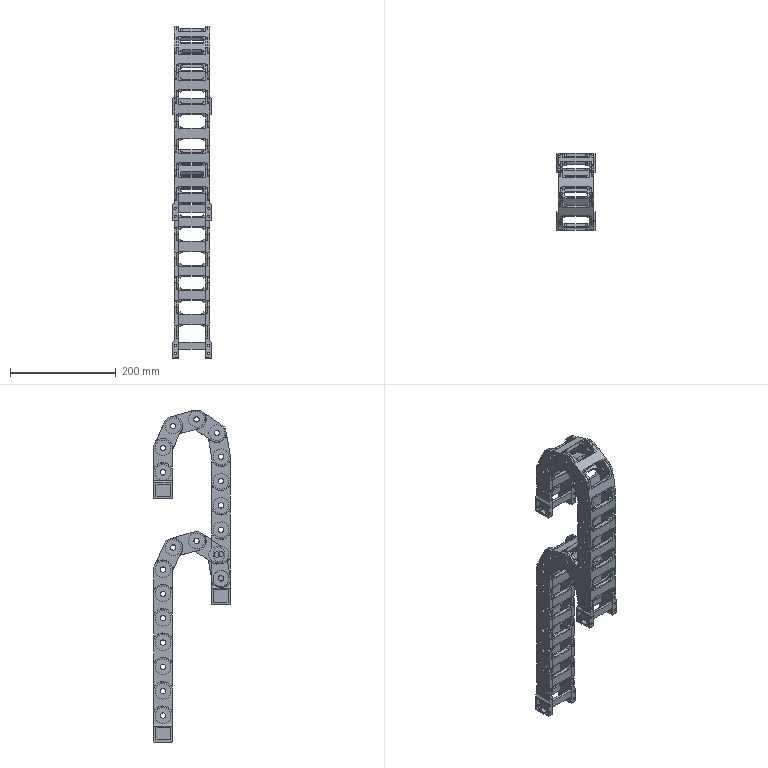Part | SolidWorks | features BaseBody 13, LPattern 4 | 23 solids | 5282 faces | volume 832857 mm3 | cylinder 2870 | plane 2412 | commonest cylinder face diameters 2 x863 4.24 x240 18.2 x172 32.34 x166 10 x160 13.7 x160